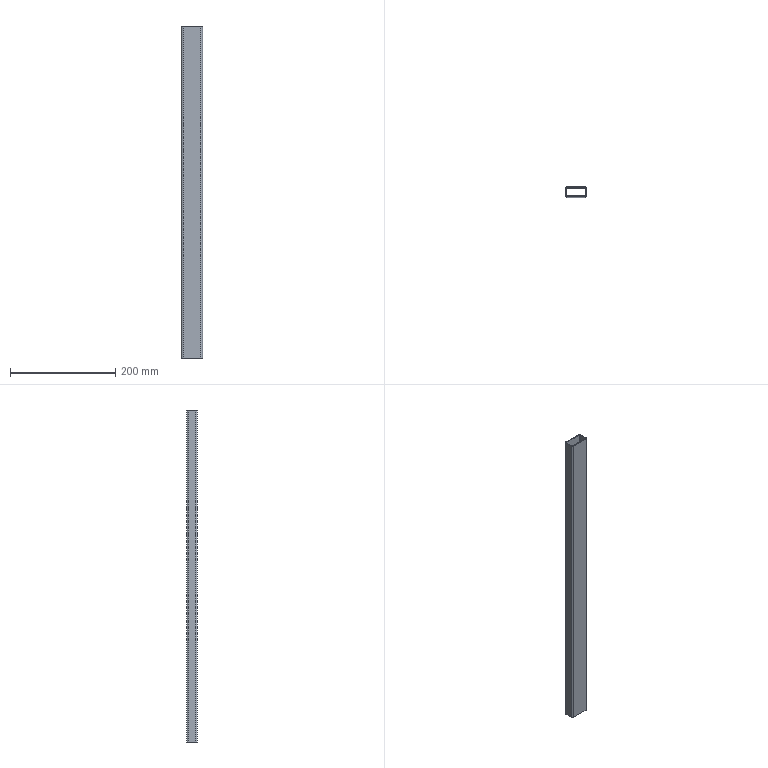Part | SolidWorks | features BaseBody 1 | 1 solid | 18 faces | box 40 x 20 x 630 mm | volume 136794 mm3 | plane 10 | cylinder 8 | commonest cylinder face diameters 2 x4 6 x4
STEP:
#1=CARTESIAN_POINT('',(18.,-7.,-315.));
#2=VERTEX_POINT('',#1);
#3=CARTESIAN_POINT('',(18.,7.,-315.));
#4=VERTEX_POINT('',#3);
#5=CARTESIAN_POINT('',(18.,7.,-315.));
#6=DIRECTION('',(0.,1.,0.));
#7=VECTOR('',#6,1000.);
#8=LINE('',#5,#7);
#9=EDGE_CURVE('',#2,#4,#8,.T.);
#10=ORIENTED_EDGE('',*,*,#9,.F.);
#11=CARTESIAN_POINT('',(18.,-7.,315.));
#12=VERTEX_POINT('',#11);
#13=CARTESIAN_POINT('',(18.,-7.,315.));
#14=DIRECTION('',(0.,0.,-1.));
#15=VECTOR('',#14,1000.);
#16=LINE('',#13,#15);
#17=EDGE_CURVE('',#12,#2,#16,.T.);
#18=ORIENTED_EDGE('',*,*,#17,.F.);
#19=CARTESIAN_POINT('',(18.,7.,315.));
#20=VERTEX_POINT('',#19);
#21=CARTESIAN_POINT('',(18.,7.,315.));
#22=DIRECTION('',(0.,1.,0.));
#23=VECTOR('',#22,1000.);
#24=LINE('',#21,#23);
#25=EDGE_CURVE('',#12,#20,#24,.T.);
#26=ORIENTED_EDGE('',*,*,#25,.T.);
#27=CARTESIAN_POINT('',(18.,7.,315.));
#28=DIRECTION('',(0.,0.,-1.));
#29=VECTOR('',#28,1000.);
#30=LINE('',#27,#29);
#31=EDGE_CURVE('',#20,#4,#30,.T.);
#32=ORIENTED_EDGE('',*,*,#31,.T.);
#33=EDGE_LOOP('',(#10,#18,#26,#32));
#34=FACE_OUTER_BOUND('',#33,.T.);
#35=CARTESIAN_POINT('',(18.,7.,315.));
#36=DIRECTION('',(-1.,0.,0.));
#37=DIRECTION('',(0.,0.,1.));
#38=AXIS2_PLACEMENT_3D('',#35,#36,#37);
#39=PLANE('',#38);
#40=ADVANCED_FACE('',(#34),#39,.T.);
#41=CARTESIAN_POINT('',(17.,-8.,-315.));
#42=VERTEX_POINT('',#41);
#43=CARTESIAN_POINT('',(17.,-7.,-315.));
#44=DIRECTION('',(0.,0.,1.));
#45=DIRECTION('',(1.,0.,0.));
#46=AXIS2_PLACEMENT_3D('',#43,#44,#45);
#47=CIRCLE('',#46,1.);
#48=EDGE_CURVE('',#42,#2,#47,.T.);
#49=ORIENTED_EDGE('',*,*,#48,.F.);
#50=CARTESIAN_POINT('',(17.,-8.,315.));
#51=VERTEX_POINT('',#50);
#52=CARTESIAN_POINT('',(17.,-8.,315.));
#53=DIRECTION('',(0.,0.,-1.));
#54=VECTOR('',#53,1000.);
#55=LINE('',#52,#54);
#56=EDGE_CURVE('',#51,#42,#55,.T.);
#57=ORIENTED_EDGE('',*,*,#56,.F.);
#58=CARTESIAN_POINT('',(17.,-7.,315.));
#59=DIRECTION('',(0.,0.,1.));
#60=DIRECTION('',(1.,0.,0.));
#61=AXIS2_PLACEMENT_3D('',#58,#59,#60);
#62=CIRCLE('',#61,1.);
#63=EDGE_CURVE('',#51,#12,#62,.T.);
#64=ORIENTED_EDGE('',*,*,#63,.T.);
#65=ORIENTED_EDGE('',*,*,#17,.T.);
#66=EDGE_LOOP('',(#49,#57,#64,#65));
#67=FACE_OUTER_BOUND('',#66,.T.);
#68=CARTESIAN_POINT('',(17.,-7.,315.));
#69=DIRECTION('',(0.,0.,-1.));
#70=DIRECTION('',(-1.,0.,0.));
#71=AXIS2_PLACEMENT_3D('',#68,#69,#70);
#72=CYLINDRICAL_SURFACE('',#71,1.);
#73=ADVANCED_FACE('',(#67),#72,.F.);
#74=CARTESIAN_POINT('',(-17.,-8.,-315.));
#75=VERTEX_POINT('',#74);
#76=CARTESIAN_POINT('',(-17.,-8.,-315.));
#77=DIRECTION('',(1.,0.,0.));
#78=VECTOR('',#77,1000.);
#79=LINE('',#76,#78);
#80=EDGE_CURVE('',#75,#42,#79,.T.);
#81=ORIENTED_EDGE('',*,*,#80,.F.);
#82=CARTESIAN_POINT('',(-17.,-8.,315.));
#83=VERTEX_POINT('',#82);
#84=CARTESIAN_POINT('',(-17.,-8.,315.));
#85=DIRECTION('',(0.,0.,-1.));
#86=VECTOR('',#85,1000.);
#87=LINE('',#84,#86);
#88=EDGE_CURVE('',#83,#75,#87,.T.);
#89=ORIENTED_EDGE('',*,*,#88,.F.);
#90=CARTESIAN_POINT('',(-17.,-8.,315.));
#91=DIRECTION('',(1.,0.,0.));
#92=VECTOR('',#91,1000.);
#93=LINE('',#90,#92);
#94=EDGE_CURVE('',#83,#51,#93,.T.);
#95=ORIENTED_EDGE('',*,*,#94,.T.);
#96=ORIENTED_EDGE('',*,*,#56,.T.);
#97=EDGE_LOOP('',(#81,#89,#95,#96));
#98=FACE_OUTER_BOUND('',#97,.T.);
#99=CARTESIAN_POINT('',(-17.,-8.,315.));
#100=DIRECTION('',(0.,1.,0.));
#101=DIRECTION('',(1.,0.,0.));
#102=AXIS2_PLACEMENT_3D('',#99,#100,#101);
#103=PLANE('',#102);
#104=ADVANCED_FACE('',(#98),#103,.T.);
#105=CARTESIAN_POINT('',(-18.,-7.,-315.));
#106=VERTEX_POINT('',#105);
#107=CARTESIAN_POINT('',(-17.,-7.,-315.));
#108=DIRECTION('',(0.,0.,1.));
#109=DIRECTION('',(1.,0.,0.));
#110=AXIS2_PLACEMENT_3D('',#107,#108,#109);
#111=CIRCLE('',#110,1.);
#112=EDGE_CURVE('',#106,#75,#111,.T.);
#113=ORIENTED_EDGE('',*,*,#112,.F.);
#114=CARTESIAN_POINT('',(-18.,-7.,315.));
#115=VERTEX_POINT('',#114);
#116=CARTESIAN_POINT('',(-18.,-7.,315.));
#117=DIRECTION('',(0.,0.,-1.));
#118=VECTOR('',#117,1000.);
#119=LINE('',#116,#118);
#120=EDGE_CURVE('',#115,#106,#119,.T.);
#121=ORIENTED_EDGE('',*,*,#120,.F.);
#122=CARTESIAN_POINT('',(-17.,-7.,315.));
#123=DIRECTION('',(0.,0.,1.));
#124=DIRECTION('',(1.,0.,0.));
#125=AXIS2_PLACEMENT_3D('',#122,#123,#124);
#126=CIRCLE('',#125,1.);
#127=EDGE_CURVE('',#115,#83,#126,.T.);
#128=ORIENTED_EDGE('',*,*,#127,.T.);
#129=ORIENTED_EDGE('',*,*,#88,.T.);
#130=EDGE_LOOP('',(#113,#121,#128,#129));
#131=FACE_OUTER_BOUND('',#130,.T.);
#132=CARTESIAN_POINT('',(-17.,-7.,315.));
#133=DIRECTION('',(0.,0.,-1.));
#134=DIRECTION('',(-1.,0.,0.));
#135=AXIS2_PLACEMENT_3D('',#132,#133,#134);
#136=CYLINDRICAL_SURFACE('',#135,1.);
#137=ADVANCED_FACE('',(#131),#136,.F.);
#138=CARTESIAN_POINT('',(-18.,7.,-315.));
#139=VERTEX_POINT('',#138);
#140=CARTESIAN_POINT('',(-18.,7.,-315.));
#141=DIRECTION('',(0.,-1.,0.));
#142=VECTOR('',#141,1000.);
#143=LINE('',#140,#142);
#144=EDGE_CURVE('',#139,#106,#143,.T.);
#145=ORIENTED_EDGE('',*,*,#144,.F.);
#146=CARTESIAN_POINT('',(-18.,7.,315.));
#147=VERTEX_POINT('',#146);
#148=CARTESIAN_POINT('',(-18.,7.,315.));
#149=DIRECTION('',(0.,0.,-1.));
#150=VECTOR('',#149,1000.);
#151=LINE('',#148,#150);
#152=EDGE_CURVE('',#147,#139,#151,.T.);
#153=ORIENTED_EDGE('',*,*,#152,.F.);
#154=CARTESIAN_POINT('',(-18.,7.,315.));
#155=DIRECTION('',(0.,-1.,0.));
#156=VECTOR('',#155,1000.);
#157=LINE('',#154,#156);
#158=EDGE_CURVE('',#147,#115,#157,.T.);
#159=ORIENTED_EDGE('',*,*,#158,.T.);
#160=ORIENTED_EDGE('',*,*,#120,.T.);
#161=EDGE_LOOP('',(#145,#153,#159,#160));
#162=FACE_OUTER_BOUND('',#161,.T.);
#163=CARTESIAN_POINT('',(-18.,7.,315.));
#164=DIRECTION('',(1.,0.,0.));
#165=DIRECTION('',(0.,-1.,0.));
#166=AXIS2_PLACEMENT_3D('',#163,#164,#165);
#167=PLANE('',#166);
#168=ADVANCED_FACE('',(#162),#167,.T.);
#169=CARTESIAN_POINT('',(-17.,8.,-315.));
#170=VERTEX_POINT('',#169);
#171=CARTESIAN_POINT('',(-17.,7.,-315.));
#172=DIRECTION('',(0.,0.,1.));
#173=DIRECTION('',(1.,0.,0.));
#174=AXIS2_PLACEMENT_3D('',#171,#172,#173);
#175=CIRCLE('',#174,1.);
#176=EDGE_CURVE('',#170,#139,#175,.T.);
#177=ORIENTED_EDGE('',*,*,#176,.F.);
#178=CARTESIAN_POINT('',(-17.,8.,315.));
#179=VERTEX_POINT('',#178);
#180=CARTESIAN_POINT('',(-17.,8.,315.));
#181=DIRECTION('',(0.,0.,-1.));
#182=VECTOR('',#181,1000.);
#183=LINE('',#180,#182);
#184=EDGE_CURVE('',#179,#170,#183,.T.);
#185=ORIENTED_EDGE('',*,*,#184,.F.);
#186=CARTESIAN_POINT('',(-17.,7.,315.));
#187=DIRECTION('',(0.,0.,1.));
#188=DIRECTION('',(1.,0.,0.));
#189=AXIS2_PLACEMENT_3D('',#186,#187,#188);
#190=CIRCLE('',#189,1.);
#191=EDGE_CURVE('',#179,#147,#190,.T.);
#192=ORIENTED_EDGE('',*,*,#191,.T.);
#193=ORIENTED_EDGE('',*,*,#152,.T.);
#194=EDGE_LOOP('',(#177,#185,#192,#193));
#195=FACE_OUTER_BOUND('',#194,.T.);
#196=CARTESIAN_POINT('',(-17.,7.,315.));
#197=DIRECTION('',(0.,0.,-1.));
#198=DIRECTION('',(-1.,0.,0.));
#199=AXIS2_PLACEMENT_3D('',#196,#197,#198);
#200=CYLINDRICAL_SURFACE('',#199,1.);
#201=ADVANCED_FACE('',(#195),#200,.F.);
#202=CARTESIAN_POINT('',(17.,8.,-315.));
#203=VERTEX_POINT('',#202);
#204=CARTESIAN_POINT('',(-17.,8.,-315.));
#205=DIRECTION('',(-1.,0.,0.));
#206=VECTOR('',#205,1000.);
#207=LINE('',#204,#206);
#208=EDGE_CURVE('',#203,#170,#207,.T.);
#209=ORIENTED_EDGE('',*,*,#208,.F.);
#210=CARTESIAN_POINT('',(17.,8.,315.));
#211=VERTEX_POINT('',#210);
#212=CARTESIAN_POINT('',(17.,8.,315.));
#213=DIRECTION('',(0.,0.,-1.));
#214=VECTOR('',#213,1000.);
#215=LINE('',#212,#214);
#216=EDGE_CURVE('',#211,#203,#215,.T.);
#217=ORIENTED_EDGE('',*,*,#216,.F.);
#218=CARTESIAN_POINT('',(-17.,8.,315.));
#219=DIRECTION('',(-1.,0.,0.));
#220=VECTOR('',#219,1000.);
#221=LINE('',#218,#220);
#222=EDGE_CURVE('',#211,#179,#221,.T.);
#223=ORIENTED_EDGE('',*,*,#222,.T.);
#224=ORIENTED_EDGE('',*,*,#184,.T.);
#225=EDGE_LOOP('',(#209,#217,#223,#224));
#226=FACE_OUTER_BOUND('',#225,.T.);
#227=CARTESIAN_POINT('',(-17.,8.,315.));
#228=DIRECTION('',(0.,-1.,0.));
#229=DIRECTION('',(0.,0.,-1.));
#230=AXIS2_PLACEMENT_3D('',#227,#228,#229);
#231=PLANE('',#230);
#232=ADVANCED_FACE('',(#226),#231,.T.);
#233=CARTESIAN_POINT('',(17.,7.,-315.));
#234=DIRECTION('',(0.,0.,1.));
#235=DIRECTION('',(-1.,0.,0.));
#236=AXIS2_PLACEMENT_3D('',#233,#234,#235);
#237=CIRCLE('',#236,1.);
#238=EDGE_CURVE('',#4,#203,#237,.T.);
#239=ORIENTED_EDGE('',*,*,#238,.F.);
#240=ORIENTED_EDGE('',*,*,#31,.F.);
#241=CARTESIAN_POINT('',(17.,7.,315.));
#242=DIRECTION('',(0.,0.,1.));
#243=DIRECTION('',(-1.,0.,0.));
#244=AXIS2_PLACEMENT_3D('',#241,#242,#243);
#245=CIRCLE('',#244,1.);
#246=EDGE_CURVE('',#20,#211,#245,.T.);
#247=ORIENTED_EDGE('',*,*,#246,.T.);
#248=ORIENTED_EDGE('',*,*,#216,.T.);
#249=EDGE_LOOP('',(#239,#240,#247,#248));
#250=FACE_OUTER_BOUND('',#249,.T.);
#251=CARTESIAN_POINT('',(17.,7.,315.));
#252=DIRECTION('',(0.,0.,-1.));
#253=DIRECTION('',(-1.,0.,0.));
#254=AXIS2_PLACEMENT_3D('',#251,#252,#253);
#255=CYLINDRICAL_SURFACE('',#254,1.);
#256=ADVANCED_FACE('',(#250),#255,.F.);
#257=CARTESIAN_POINT('',(-17.,-10.,-315.));
#258=VERTEX_POINT('',#257);
#259=CARTESIAN_POINT('',(17.,-10.,-315.));
#260=VERTEX_POINT('',#259);
#261=CARTESIAN_POINT('',(-17.,-10.,-315.));
#262=DIRECTION('',(1.,0.,0.));
#263=VECTOR('',#262,1000.);
#264=LINE('',#261,#263);
#265=EDGE_CURVE('',#258,#260,#264,.T.);
#266=ORIENTED_EDGE('',*,*,#265,.T.);
#267=CARTESIAN_POINT('',(17.,-10.,315.));
#268=VERTEX_POINT('',#267);
#269=CARTESIAN_POINT('',(17.,-10.,315.));
#270=DIRECTION('',(0.,0.,-1.));
#271=VECTOR('',#270,1000.);
#272=LINE('',#269,#271);
#273=EDGE_CURVE('',#268,#260,#272,.T.);
#274=ORIENTED_EDGE('',*,*,#273,.F.);
#275=CARTESIAN_POINT('',(-17.,-10.,315.));
#276=VERTEX_POINT('',#275);
#277=CARTESIAN_POINT('',(-17.,-10.,315.));
#278=DIRECTION('',(1.,0.,0.));
#279=VECTOR('',#278,1000.);
#280=LINE('',#277,#279);
#281=EDGE_CURVE('',#276,#268,#280,.T.);
#282=ORIENTED_EDGE('',*,*,#281,.F.);
#283=CARTESIAN_POINT('',(-17.,-10.,315.));
#284=DIRECTION('',(0.,0.,-1.));
#285=VECTOR('',#284,1000.);
#286=LINE('',#283,#285);
#287=EDGE_CURVE('',#276,#258,#286,.T.);
#288=ORIENTED_EDGE('',*,*,#287,.T.);
#289=EDGE_LOOP('',(#266,#274,#282,#288));
#290=FACE_OUTER_BOUND('',#289,.T.);
#291=CARTESIAN_POINT('',(-17.,-10.,315.));
#292=DIRECTION('',(0.,1.,0.));
#293=DIRECTION('',(1.,0.,0.));
#294=AXIS2_PLACEMENT_3D('',#291,#292,#293);
#295=PLANE('',#294);
#296=ADVANCED_FACE('',(#290),#295,.F.);
#297=CARTESIAN_POINT('',(-20.,-7.,-315.));
#298=VERTEX_POINT('',#297);
#299=CARTESIAN_POINT('',(-17.,-7.,-315.));
#300=DIRECTION('',(0.,0.,1.));
#301=DIRECTION('',(1.,0.,0.));
#302=AXIS2_PLACEMENT_3D('',#299,#300,#301);
#303=CIRCLE('',#302,3.);
#304=EDGE_CURVE('',#298,#258,#303,.T.);
#305=ORIENTED_EDGE('',*,*,#304,.T.);
#306=ORIENTED_EDGE('',*,*,#287,.F.);
#307=CARTESIAN_POINT('',(-20.,-7.,315.));
#308=VERTEX_POINT('',#307);
#309=CARTESIAN_POINT('',(-17.,-7.,315.));
#310=DIRECTION('',(0.,0.,1.));
#311=DIRECTION('',(1.,0.,0.));
#312=AXIS2_PLACEMENT_3D('',#309,#310,#311);
#313=CIRCLE('',#312,3.);
#314=EDGE_CURVE('',#308,#276,#313,.T.);
#315=ORIENTED_EDGE('',*,*,#314,.F.);
#316=CARTESIAN_POINT('',(-20.,-7.,315.));
#317=DIRECTION('',(0.,0.,-1.));
#318=VECTOR('',#317,1000.);
#319=LINE('',#316,#318);
#320=EDGE_CURVE('',#308,#298,#319,.T.);
#321=ORIENTED_EDGE('',*,*,#320,.T.);
#322=EDGE_LOOP('',(#305,#306,#315,#321));
#323=FACE_OUTER_BOUND('',#322,.T.);
#324=CARTESIAN_POINT('',(-17.,-7.,315.));
#325=DIRECTION('',(0.,0.,-1.));
#326=DIRECTION('',(-1.,0.,0.));
#327=AXIS2_PLACEMENT_3D('',#324,#325,#326);
#328=CYLINDRICAL_SURFACE('',#327,3.);
#329=ADVANCED_FACE('',(#323),#328,.T.);
#330=CARTESIAN_POINT('',(-20.,7.,-315.));
#331=VERTEX_POINT('',#330);
#332=CARTESIAN_POINT('',(-20.,7.,-315.));
#333=DIRECTION('',(0.,-1.,0.));
#334=VECTOR('',#333,1000.);
#335=LINE('',#332,#334);
#336=EDGE_CURVE('',#331,#298,#335,.T.);
#337=ORIENTED_EDGE('',*,*,#336,.T.);
#338=ORIENTED_EDGE('',*,*,#320,.F.);
#339=CARTESIAN_POINT('',(-20.,7.,315.));
#340=VERTEX_POINT('',#339);
#341=CARTESIAN_POINT('',(-20.,7.,315.));
#342=DIRECTION('',(0.,-1.,0.));
#343=VECTOR('',#342,1000.);
#344=LINE('',#341,#343);
#345=EDGE_CURVE('',#340,#308,#344,.T.);
#346=ORIENTED_EDGE('',*,*,#345,.F.);
#347=CARTESIAN_POINT('',(-20.,7.,315.));
#348=DIRECTION('',(0.,0.,-1.));
#349=VECTOR('',#348,1000.);
#350=LINE('',#347,#349);
#351=EDGE_CURVE('',#340,#331,#350,.T.);
#352=ORIENTED_EDGE('',*,*,#351,.T.);
#353=EDGE_LOOP('',(#337,#338,#346,#352));
#354=FACE_OUTER_BOUND('',#353,.T.);
#355=CARTESIAN_POINT('',(-20.,7.,315.));
#356=DIRECTION('',(1.,0.,0.));
#357=DIRECTION('',(0.,1.,0.));
#358=AXIS2_PLACEMENT_3D('',#355,#356,#357);
#359=PLANE('',#358);
#360=ADVANCED_FACE('',(#354),#359,.F.);
#361=CARTESIAN_POINT('',(-17.,10.,-315.));
#362=VERTEX_POINT('',#361);
#363=CARTESIAN_POINT('',(-17.,7.,-315.));
#364=DIRECTION('',(0.,0.,1.));
#365=DIRECTION('',(1.,0.,0.));
#366=AXIS2_PLACEMENT_3D('',#363,#364,#365);
#367=CIRCLE('',#366,3.);
#368=EDGE_CURVE('',#362,#331,#367,.T.);
#369=ORIENTED_EDGE('',*,*,#368,.T.);
#370=ORIENTED_EDGE('',*,*,#351,.F.);
#371=CARTESIAN_POINT('',(-17.,10.,315.));
#372=VERTEX_POINT('',#371);
#373=CARTESIAN_POINT('',(-17.,7.,315.));
#374=DIRECTION('',(0.,0.,1.));
#375=DIRECTION('',(1.,0.,0.));
#376=AXIS2_PLACEMENT_3D('',#373,#374,#375);
#377=CIRCLE('',#376,3.);
#378=EDGE_CURVE('',#372,#340,#377,.T.);
#379=ORIENTED_EDGE('',*,*,#378,.F.);
#380=CARTESIAN_POINT('',(-17.,10.,315.));
#381=DIRECTION('',(0.,0.,-1.));
#382=VECTOR('',#381,1000.);
#383=LINE('',#380,#382);
#384=EDGE_CURVE('',#372,#362,#383,.T.);
#385=ORIENTED_EDGE('',*,*,#384,.T.);
#386=EDGE_LOOP('',(#369,#370,#379,#385));
#387=FACE_OUTER_BOUND('',#386,.T.);
#388=CARTESIAN_POINT('',(-17.,7.,315.));
#389=DIRECTION('',(0.,0.,-1.));
#390=DIRECTION('',(-1.,0.,0.));
#391=AXIS2_PLACEMENT_3D('',#388,#389,#390);
#392=CYLINDRICAL_SURFACE('',#391,3.);
#393=ADVANCED_FACE('',(#387),#392,.T.);
#394=CARTESIAN_POINT('',(17.,10.,-315.));
#395=VERTEX_POINT('',#394);
#396=CARTESIAN_POINT('',(-17.,10.,-315.));
#397=DIRECTION('',(-1.,0.,0.));
#398=VECTOR('',#397,1000.);
#399=LINE('',#396,#398);
#400=EDGE_CURVE('',#395,#362,#399,.T.);
#401=ORIENTED_EDGE('',*,*,#400,.T.);
#402=ORIENTED_EDGE('',*,*,#384,.F.);
#403=CARTESIAN_POINT('',(17.,10.,315.));
#404=VERTEX_POINT('',#403);
#405=CARTESIAN_POINT('',(-17.,10.,315.));
#406=DIRECTION('',(-1.,0.,0.));
#407=VECTOR('',#406,1000.);
#408=LINE('',#405,#407);
#409=EDGE_CURVE('',#404,#372,#408,.T.);
#410=ORIENTED_EDGE('',*,*,#409,.F.);
#411=CARTESIAN_POINT('',(17.,10.,315.));
#412=DIRECTION('',(0.,0.,-1.));
#413=VECTOR('',#412,1000.);
#414=LINE('',#411,#413);
#415=EDGE_CURVE('',#404,#395,#414,.T.);
#416=ORIENTED_EDGE('',*,*,#415,.T.);
#417=EDGE_LOOP('',(#401,#402,#410,#416));
#418=FACE_OUTER_BOUND('',#417,.T.);
#419=CARTESIAN_POINT('',(-17.,10.,315.));
#420=DIRECTION('',(0.,-1.,0.));
#421=DIRECTION('',(0.,0.,-1.));
#422=AXIS2_PLACEMENT_3D('',#419,#420,#421);
#423=PLANE('',#422);
#424=ADVANCED_FACE('',(#418),#423,.F.);
#425=CARTESIAN_POINT('',(20.,7.,-315.));
#426=VERTEX_POINT('',#425);
#427=CARTESIAN_POINT('',(17.,7.,-315.));
#428=DIRECTION('',(0.,0.,1.));
#429=DIRECTION('',(-1.,0.,0.));
#430=AXIS2_PLACEMENT_3D('',#427,#428,#429);
#431=CIRCLE('',#430,3.);
#432=EDGE_CURVE('',#426,#395,#431,.T.);
#433=ORIENTED_EDGE('',*,*,#432,.T.);
#434=ORIENTED_EDGE('',*,*,#415,.F.);
#435=CARTESIAN_POINT('',(20.,7.,315.));
#436=VERTEX_POINT('',#435);
#437=CARTESIAN_POINT('',(17.,7.,315.));
#438=DIRECTION('',(0.,0.,1.));
#439=DIRECTION('',(-1.,0.,0.));
#440=AXIS2_PLACEMENT_3D('',#437,#438,#439);
#441=CIRCLE('',#440,3.);
#442=EDGE_CURVE('',#436,#404,#441,.T.);
#443=ORIENTED_EDGE('',*,*,#442,.F.);
#444=CARTESIAN_POINT('',(20.,7.,315.));
#445=DIRECTION('',(0.,0.,-1.));
#446=VECTOR('',#445,1000.);
#447=LINE('',#444,#446);
#448=EDGE_CURVE('',#436,#426,#447,.T.);
#449=ORIENTED_EDGE('',*,*,#448,.T.);
#450=EDGE_LOOP('',(#433,#434,#443,#449));
#451=FACE_OUTER_BOUND('',#450,.T.);
#452=CARTESIAN_POINT('',(17.,7.,315.));
#453=DIRECTION('',(0.,0.,-1.));
#454=DIRECTION('',(-1.,0.,0.));
#455=AXIS2_PLACEMENT_3D('',#452,#453,#454);
#456=CYLINDRICAL_SURFACE('',#455,3.);
#457=ADVANCED_FACE('',(#451),#456,.T.);
#458=CARTESIAN_POINT('',(20.,-7.,-315.));
#459=VERTEX_POINT('',#458);
#460=CARTESIAN_POINT('',(20.,7.,-315.));
#461=DIRECTION('',(0.,1.,0.));
#462=VECTOR('',#461,1000.);
#463=LINE('',#460,#462);
#464=EDGE_CURVE('',#459,#426,#463,.T.);
#465=ORIENTED_EDGE('',*,*,#464,.T.);
#466=ORIENTED_EDGE('',*,*,#448,.F.);
#467=CARTESIAN_POINT('',(20.,-7.,315.));
#468=VERTEX_POINT('',#467);
#469=CARTESIAN_POINT('',(20.,7.,315.));
#470=DIRECTION('',(0.,1.,0.));
#471=VECTOR('',#470,1000.);
#472=LINE('',#469,#471);
#473=EDGE_CURVE('',#468,#436,#472,.T.);
#474=ORIENTED_EDGE('',*,*,#473,.F.);
#475=CARTESIAN_POINT('',(20.,-7.,315.));
#476=DIRECTION('',(0.,0.,-1.));
#477=VECTOR('',#476,1000.);
#478=LINE('',#475,#477);
#479=EDGE_CURVE('',#468,#459,#478,.T.);
#480=ORIENTED_EDGE('',*,*,#479,.T.);
#481=EDGE_LOOP('',(#465,#466,#474,#480));
#482=FACE_OUTER_BOUND('',#481,.T.);
#483=CARTESIAN_POINT('',(20.,7.,315.));
#484=DIRECTION('',(-1.,0.,0.));
#485=DIRECTION('',(0.,0.,1.));
#486=AXIS2_PLACEMENT_3D('',#483,#484,#485);
#487=PLANE('',#486);
#488=ADVANCED_FACE('',(#482),#487,.F.);
#489=CARTESIAN_POINT('',(17.,-7.,-315.));
#490=DIRECTION('',(0.,0.,1.));
#491=DIRECTION('',(1.,0.,0.));
#492=AXIS2_PLACEMENT_3D('',#489,#490,#491);
#493=CIRCLE('',#492,3.);
#494=EDGE_CURVE('',#260,#459,#493,.T.);
#495=ORIENTED_EDGE('',*,*,#494,.T.);
#496=ORIENTED_EDGE('',*,*,#479,.F.);
#497=CARTESIAN_POINT('',(17.,-7.,315.));
#498=DIRECTION('',(0.,0.,1.));
#499=DIRECTION('',(1.,0.,0.));
#500=AXIS2_PLACEMENT_3D('',#497,#498,#499);
#501=CIRCLE('',#500,3.);
#502=EDGE_CURVE('',#268,#468,#501,.T.);
#503=ORIENTED_EDGE('',*,*,#502,.F.);
#504=ORIENTED_EDGE('',*,*,#273,.T.);
#505=EDGE_LOOP('',(#495,#496,#503,#504));
#506=FACE_OUTER_BOUND('',#505,.T.);
#507=CARTESIAN_POINT('',(17.,-7.,315.));
#508=DIRECTION('',(0.,0.,-1.));
#509=DIRECTION('',(-1.,0.,0.));
#510=AXIS2_PLACEMENT_3D('',#507,#508,#509);
#511=CYLINDRICAL_SURFACE('',#510,3.);
#512=ADVANCED_FACE('',(#506),#511,.T.);
#513=ORIENTED_EDGE('',*,*,#238,.T.);
#514=ORIENTED_EDGE('',*,*,#208,.T.);
#515=ORIENTED_EDGE('',*,*,#176,.T.);
#516=ORIENTED_EDGE('',*,*,#144,.T.);
#517=ORIENTED_EDGE('',*,*,#112,.T.);
#518=ORIENTED_EDGE('',*,*,#80,.T.);
#519=ORIENTED_EDGE('',*,*,#48,.T.);
#520=ORIENTED_EDGE('',*,*,#9,.T.);
#521=EDGE_LOOP('',(#513,#514,#515,#516,#517,#518,#519,#520));
#522=FACE_BOUND('',#521,.T.);
#523=ORIENTED_EDGE('',*,*,#494,.F.);
#524=ORIENTED_EDGE('',*,*,#265,.F.);
#525=ORIENTED_EDGE('',*,*,#304,.F.);
#526=ORIENTED_EDGE('',*,*,#336,.F.);
#527=ORIENTED_EDGE('',*,*,#368,.F.);
#528=ORIENTED_EDGE('',*,*,#400,.F.);
#529=ORIENTED_EDGE('',*,*,#432,.F.);
#530=ORIENTED_EDGE('',*,*,#464,.F.);
#531=EDGE_LOOP('',(#523,#524,#525,#526,#527,#528,#529,#530));
#532=FACE_OUTER_BOUND('',#531,.T.);
#533=CARTESIAN_POINT('',(17.,-7.,-315.));
#534=DIRECTION('',(0.,0.,1.));
#535=DIRECTION('',(1.,0.,0.));
#536=AXIS2_PLACEMENT_3D('',#533,#534,#535);
#537=PLANE('',#536);
#538=ADVANCED_FACE('',(#522,#532),#537,.F.);
#539=ORIENTED_EDGE('',*,*,#222,.F.);
#540=ORIENTED_EDGE('',*,*,#246,.F.);
#541=ORIENTED_EDGE('',*,*,#25,.F.);
#542=ORIENTED_EDGE('',*,*,#63,.F.);
#543=ORIENTED_EDGE('',*,*,#94,.F.);
#544=ORIENTED_EDGE('',*,*,#127,.F.);
#545=ORIENTED_EDGE('',*,*,#158,.F.);
#546=ORIENTED_EDGE('',*,*,#191,.F.);
#547=EDGE_LOOP('',(#539,#540,#541,#542,#543,#544,#545,#546));
#548=FACE_BOUND('',#547,.T.);
#549=ORIENTED_EDGE('',*,*,#502,.T.);
#550=ORIENTED_EDGE('',*,*,#473,.T.);
#551=ORIENTED_EDGE('',*,*,#442,.T.);
#552=ORIENTED_EDGE('',*,*,#409,.T.);
#553=ORIENTED_EDGE('',*,*,#378,.T.);
#554=ORIENTED_EDGE('',*,*,#345,.T.);
#555=ORIENTED_EDGE('',*,*,#314,.T.);
#556=ORIENTED_EDGE('',*,*,#281,.T.);
#557=EDGE_LOOP('',(#549,#550,#551,#552,#553,#554,#555,#556));
#558=FACE_OUTER_BOUND('',#557,.T.);
#559=CARTESIAN_POINT('',(17.,-7.,315.));
#560=DIRECTION('',(0.,0.,1.));
#561=DIRECTION('',(1.,0.,0.));
#562=AXIS2_PLACEMENT_3D('',#559,#560,#561);
#563=PLANE('',#562);
#564=ADVANCED_FACE('',(#548,#558),#563,.T.);
#565=CLOSED_SHELL('',(#40,#73,#104,#137,#168,#201,#232,#256,#296,#329,#360,#393,#424,#457,#488,#512,#538,#564));
#566=MANIFOLD_SOLID_BREP('',#565);
#567=CARTESIAN_POINT('',(0.,0.,0.));
#568=DIRECTION('',(0.,0.,1.));
#569=DIRECTION('',(1.,0.,0.));
#570=AXIS2_PLACEMENT_3D('',#567,#568,#569);
#571=(LENGTH_UNIT()NAMED_UNIT(*)SI_UNIT(.MILLI.,.METRE.));
#572=UNCERTAINTY_MEASURE_WITH_UNIT(LENGTH_MEASURE(0.00001),#571,'','');
#573=(NAMED_UNIT(*)PLANE_ANGLE_UNIT()SI_UNIT($,.RADIAN.));
#574=(NAMED_UNIT(*)SI_UNIT($,.STERADIAN.)SOLID_ANGLE_UNIT());
#575=(GEOMETRIC_REPRESENTATION_CONTEXT(3)GLOBAL_UNCERTAINTY_ASSIGNED_CONTEXT((#572))GLOBAL_UNIT_ASSIGNED_CONTEXT((#571,#573,#574))REPRESENTATION_CONTEXT('',''));
#576=ADVANCED_BREP_SHAPE_REPRESENTATION('',(#566,#570),#575);